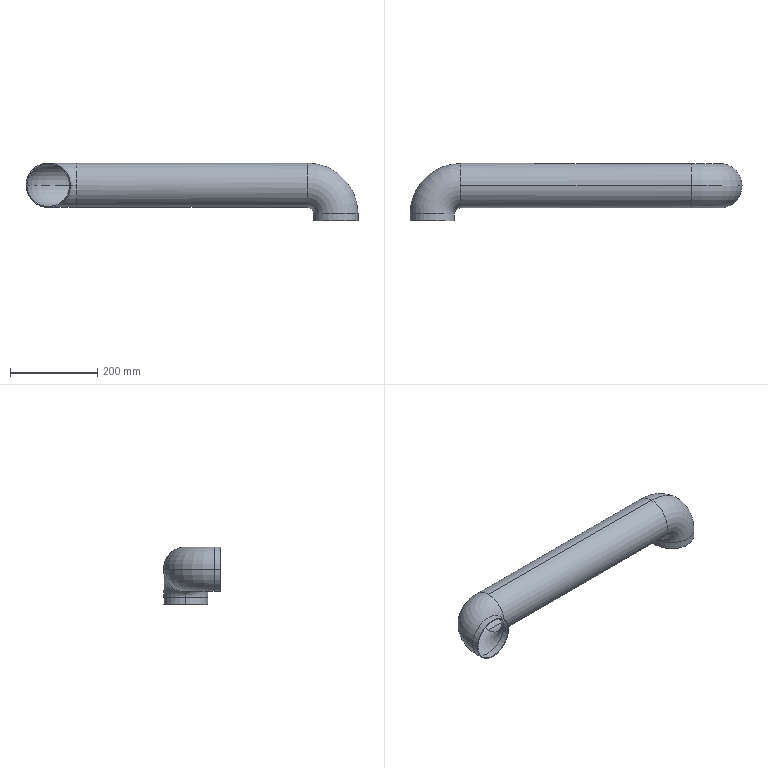Part | SolidWorks | features BaseBody 1 | 1 solid | 22 faces | box 761.5 x 131 x 133 mm | volume 481106 mm3 | cylinder 12 | torus 8 | plane 2 | commonest cylinder face diameters 98 x6 102 x6
STEP:
#1=CARTESIAN_POINT('',(65.,80.,51.));
#2=VERTEX_POINT('',#1);
#3=CARTESIAN_POINT('',(65.,131.,0.));
#4=VERTEX_POINT('',#3);
#5=CARTESIAN_POINT('',(65.,80.,0.));
#6=DIRECTION('',(-1.,0.,0.));
#7=DIRECTION('',(0.,0.,1.));
#8=AXIS2_PLACEMENT_3D('',#5,#6,#7);
#9=CIRCLE('',#8,51.);
#10=EDGE_CURVE('',#2,#4,#9,.T.);
#11=ORIENTED_EDGE('',*,*,#10,.T.);
#12=CARTESIAN_POINT('',(-51.,15.,0.));
#13=VERTEX_POINT('',#12);
#14=CARTESIAN_POINT('',(65.,15.,0.));
#15=DIRECTION('',(0.,0.,1.));
#16=DIRECTION('',(1.,0.,0.));
#17=AXIS2_PLACEMENT_3D('',#14,#15,#16);
#18=CIRCLE('',#17,116.);
#19=EDGE_CURVE('',#4,#13,#18,.T.);
#20=ORIENTED_EDGE('',*,*,#19,.T.);
#21=CARTESIAN_POINT('',(51.,15.,0.));
#22=VERTEX_POINT('',#21);
#23=CARTESIAN_POINT('',(0.,15.,0.));
#24=DIRECTION('',(0.,-1.,0.));
#25=DIRECTION('',(0.,0.,1.));
#26=AXIS2_PLACEMENT_3D('',#23,#24,#25);
#27=CIRCLE('',#26,51.);
#28=EDGE_CURVE('',#22,#13,#27,.T.);
#29=ORIENTED_EDGE('',*,*,#28,.F.);
#30=CARTESIAN_POINT('',(65.,29.,0.));
#31=VERTEX_POINT('',#30);
#32=CARTESIAN_POINT('',(65.,15.,0.));
#33=DIRECTION('',(0.,0.,1.));
#34=DIRECTION('',(1.,0.,0.));
#35=AXIS2_PLACEMENT_3D('',#32,#33,#34);
#36=CIRCLE('',#35,14.);
#37=EDGE_CURVE('',#31,#22,#36,.T.);
#38=ORIENTED_EDGE('',*,*,#37,.F.);
#39=CARTESIAN_POINT('',(65.,80.,0.));
#40=DIRECTION('',(-1.,0.,0.));
#41=DIRECTION('',(0.,0.,1.));
#42=AXIS2_PLACEMENT_3D('',#39,#40,#41);
#43=CIRCLE('',#42,51.);
#44=EDGE_CURVE('',#31,#2,#43,.T.);
#45=ORIENTED_EDGE('',*,*,#44,.T.);
#46=EDGE_LOOP('',(#11,#20,#29,#38,#45));
#47=FACE_OUTER_BOUND('',#46,.T.);
#48=CARTESIAN_POINT('',(65.,15.,0.));
#49=DIRECTION('',(0.,0.,1.));
#50=DIRECTION('',(1.,0.,0.));
#51=AXIS2_PLACEMENT_3D('',#48,#49,#50);
#52=TOROIDAL_SURFACE('',#51,65.,51.);
#53=ADVANCED_FACE('',(#47),#52,.T.);
#54=CARTESIAN_POINT('',(65.,129.,0.));
#55=VERTEX_POINT('',#54);
#56=CARTESIAN_POINT('',(65.,80.,-49.));
#57=VERTEX_POINT('',#56);
#58=CARTESIAN_POINT('',(65.,80.,0.));
#59=DIRECTION('',(-1.,0.,0.));
#60=DIRECTION('',(0.,0.,1.));
#61=AXIS2_PLACEMENT_3D('',#58,#59,#60);
#62=CIRCLE('',#61,49.);
#63=EDGE_CURVE('',#55,#57,#62,.T.);
#64=ORIENTED_EDGE('',*,*,#63,.F.);
#65=CARTESIAN_POINT('',(-49.,15.,0.));
#66=VERTEX_POINT('',#65);
#67=CARTESIAN_POINT('',(65.,15.,0.));
#68=DIRECTION('',(0.,0.,1.));
#69=DIRECTION('',(1.,0.,0.));
#70=AXIS2_PLACEMENT_3D('',#67,#68,#69);
#71=CIRCLE('',#70,114.);
#72=EDGE_CURVE('',#55,#66,#71,.T.);
#73=ORIENTED_EDGE('',*,*,#72,.T.);
#74=CARTESIAN_POINT('',(49.,15.,0.));
#75=VERTEX_POINT('',#74);
#76=CARTESIAN_POINT('',(0.,15.,0.));
#77=DIRECTION('',(0.,-1.,0.));
#78=DIRECTION('',(0.,0.,1.));
#79=AXIS2_PLACEMENT_3D('',#76,#77,#78);
#80=CIRCLE('',#79,49.);
#81=EDGE_CURVE('',#66,#75,#80,.T.);
#82=ORIENTED_EDGE('',*,*,#81,.T.);
#83=CARTESIAN_POINT('',(65.,31.,0.));
#84=VERTEX_POINT('',#83);
#85=CARTESIAN_POINT('',(65.,15.,0.));
#86=DIRECTION('',(0.,0.,1.));
#87=DIRECTION('',(1.,0.,0.));
#88=AXIS2_PLACEMENT_3D('',#85,#86,#87);
#89=CIRCLE('',#88,16.);
#90=EDGE_CURVE('',#84,#75,#89,.T.);
#91=ORIENTED_EDGE('',*,*,#90,.F.);
#92=CARTESIAN_POINT('',(65.,80.,0.));
#93=DIRECTION('',(-1.,0.,0.));
#94=DIRECTION('',(0.,0.,1.));
#95=AXIS2_PLACEMENT_3D('',#92,#93,#94);
#96=CIRCLE('',#95,49.);
#97=EDGE_CURVE('',#57,#84,#96,.T.);
#98=ORIENTED_EDGE('',*,*,#97,.F.);
#99=EDGE_LOOP('',(#64,#73,#82,#91,#98));
#100=FACE_OUTER_BOUND('',#99,.T.);
#101=CARTESIAN_POINT('',(65.,15.,0.));
#102=DIRECTION('',(0.,0.,1.));
#103=DIRECTION('',(1.,0.,0.));
#104=AXIS2_PLACEMENT_3D('',#101,#102,#103);
#105=TOROIDAL_SURFACE('',#104,65.,49.);
#106=ADVANCED_FACE('',(#100),#105,.F.);
#107=CARTESIAN_POINT('',(608.5,80.,-65.));
#108=VERTEX_POINT('',#107);
#109=CARTESIAN_POINT('',(710.5,80.,-65.));
#110=VERTEX_POINT('',#109);
#111=CARTESIAN_POINT('',(659.5,80.,-65.));
#112=DIRECTION('',(0.,0.,1.));
#113=DIRECTION('',(1.,0.,0.));
#114=AXIS2_PLACEMENT_3D('',#111,#112,#113);
#115=CIRCLE('',#114,51.);
#116=EDGE_CURVE('',#108,#110,#115,.T.);
#117=ORIENTED_EDGE('',*,*,#116,.T.);
#118=CARTESIAN_POINT('',(594.5,80.,51.));
#119=VERTEX_POINT('',#118);
#120=CARTESIAN_POINT('',(594.5,80.,-65.));
#121=DIRECTION('',(0.,-1.,0.));
#122=DIRECTION('',(0.,0.,-1.));
#123=AXIS2_PLACEMENT_3D('',#120,#121,#122);
#124=CIRCLE('',#123,116.);
#125=EDGE_CURVE('',#110,#119,#124,.T.);
#126=ORIENTED_EDGE('',*,*,#125,.T.);
#127=CARTESIAN_POINT('',(594.5,80.,-51.));
#128=VERTEX_POINT('',#127);
#129=CARTESIAN_POINT('',(594.5,80.,0.));
#130=DIRECTION('',(-1.,0.,0.));
#131=DIRECTION('',(0.,0.,1.));
#132=AXIS2_PLACEMENT_3D('',#129,#130,#131);
#133=CIRCLE('',#132,51.);
#134=EDGE_CURVE('',#128,#119,#133,.T.);
#135=ORIENTED_EDGE('',*,*,#134,.F.);
#136=CARTESIAN_POINT('',(594.5,80.,-65.));
#137=DIRECTION('',(0.,-1.,0.));
#138=DIRECTION('',(0.,0.,-1.));
#139=AXIS2_PLACEMENT_3D('',#136,#137,#138);
#140=CIRCLE('',#139,14.);
#141=EDGE_CURVE('',#108,#128,#140,.T.);
#142=ORIENTED_EDGE('',*,*,#141,.F.);
#143=EDGE_LOOP('',(#117,#126,#135,#142));
#144=FACE_OUTER_BOUND('',#143,.T.);
#145=CARTESIAN_POINT('',(594.5,80.,-65.));
#146=DIRECTION('',(0.,-1.,0.));
#147=DIRECTION('',(0.,0.,-1.));
#148=AXIS2_PLACEMENT_3D('',#145,#146,#147);
#149=TOROIDAL_SURFACE('',#148,65.,51.);
#150=ADVANCED_FACE('',(#144),#149,.T.);
#151=CARTESIAN_POINT('',(708.5,80.,-65.));
#152=VERTEX_POINT('',#151);
#153=CARTESIAN_POINT('',(610.5,80.,-65.));
#154=VERTEX_POINT('',#153);
#155=CARTESIAN_POINT('',(659.5,80.,-65.));
#156=DIRECTION('',(0.,0.,1.));
#157=DIRECTION('',(1.,0.,0.));
#158=AXIS2_PLACEMENT_3D('',#155,#156,#157);
#159=CIRCLE('',#158,49.);
#160=EDGE_CURVE('',#152,#154,#159,.T.);
#161=ORIENTED_EDGE('',*,*,#160,.F.);
#162=CARTESIAN_POINT('',(594.5,80.,49.));
#163=VERTEX_POINT('',#162);
#164=CARTESIAN_POINT('',(594.5,80.,-65.));
#165=DIRECTION('',(0.,-1.,0.));
#166=DIRECTION('',(0.,0.,-1.));
#167=AXIS2_PLACEMENT_3D('',#164,#165,#166);
#168=CIRCLE('',#167,114.);
#169=EDGE_CURVE('',#152,#163,#168,.T.);
#170=ORIENTED_EDGE('',*,*,#169,.T.);
#171=CARTESIAN_POINT('',(594.5,80.,-49.));
#172=VERTEX_POINT('',#171);
#173=CARTESIAN_POINT('',(594.5,80.,0.));
#174=DIRECTION('',(-1.,0.,0.));
#175=DIRECTION('',(0.,0.,1.));
#176=AXIS2_PLACEMENT_3D('',#173,#174,#175);
#177=CIRCLE('',#176,49.);
#178=EDGE_CURVE('',#163,#172,#177,.T.);
#179=ORIENTED_EDGE('',*,*,#178,.T.);
#180=CARTESIAN_POINT('',(594.5,80.,-65.));
#181=DIRECTION('',(0.,-1.,0.));
#182=DIRECTION('',(0.,0.,-1.));
#183=AXIS2_PLACEMENT_3D('',#180,#181,#182);
#184=CIRCLE('',#183,16.);
#185=EDGE_CURVE('',#154,#172,#184,.T.);
#186=ORIENTED_EDGE('',*,*,#185,.F.);
#187=EDGE_LOOP('',(#161,#170,#179,#186));
#188=FACE_OUTER_BOUND('',#187,.T.);
#189=CARTESIAN_POINT('',(594.5,80.,-65.));
#190=DIRECTION('',(0.,-1.,0.));
#191=DIRECTION('',(0.,0.,-1.));
#192=AXIS2_PLACEMENT_3D('',#189,#190,#191);
#193=TOROIDAL_SURFACE('',#192,65.,49.);
#194=ADVANCED_FACE('',(#188),#193,.F.);
#195=ORIENTED_EDGE('',*,*,#28,.T.);
#196=CARTESIAN_POINT('',(-51.,0.,0.));
#197=VERTEX_POINT('',#196);
#198=CARTESIAN_POINT('',(-51.,15.,0.));
#199=DIRECTION('',(0.,-1.,0.));
#200=VECTOR('',#199,1000.);
#201=LINE('',#198,#200);
#202=EDGE_CURVE('',#13,#197,#201,.T.);
#203=ORIENTED_EDGE('',*,*,#202,.T.);
#204=CARTESIAN_POINT('',(51.,0.,0.));
#205=VERTEX_POINT('',#204);
#206=CARTESIAN_POINT('',(0.,0.,0.));
#207=DIRECTION('',(0.,-1.,0.));
#208=DIRECTION('',(0.,0.,1.));
#209=AXIS2_PLACEMENT_3D('',#206,#207,#208);
#210=CIRCLE('',#209,51.);
#211=EDGE_CURVE('',#205,#197,#210,.T.);
#212=ORIENTED_EDGE('',*,*,#211,.F.);
#213=CARTESIAN_POINT('',(51.,15.,0.));
#214=DIRECTION('',(0.,-1.,0.));
#215=VECTOR('',#214,1000.);
#216=LINE('',#213,#215);
#217=EDGE_CURVE('',#22,#205,#216,.T.);
#218=ORIENTED_EDGE('',*,*,#217,.F.);
#219=EDGE_LOOP('',(#195,#203,#212,#218));
#220=FACE_OUTER_BOUND('',#219,.T.);
#221=CARTESIAN_POINT('',(0.,15.,0.));
#222=DIRECTION('',(0.,-1.,0.));
#223=DIRECTION('',(1.,0.,0.));
#224=AXIS2_PLACEMENT_3D('',#221,#222,#223);
#225=CYLINDRICAL_SURFACE('',#224,51.);
#226=ADVANCED_FACE('',(#220),#225,.T.);
#227=ORIENTED_EDGE('',*,*,#81,.F.);
#228=CARTESIAN_POINT('',(-49.,0.,0.));
#229=VERTEX_POINT('',#228);
#230=CARTESIAN_POINT('',(-49.,15.,0.));
#231=DIRECTION('',(0.,-1.,0.));
#232=VECTOR('',#231,1000.);
#233=LINE('',#230,#232);
#234=EDGE_CURVE('',#66,#229,#233,.T.);
#235=ORIENTED_EDGE('',*,*,#234,.T.);
#236=CARTESIAN_POINT('',(49.,0.,0.));
#237=VERTEX_POINT('',#236);
#238=CARTESIAN_POINT('',(0.,0.,0.));
#239=DIRECTION('',(0.,-1.,0.));
#240=DIRECTION('',(0.,0.,1.));
#241=AXIS2_PLACEMENT_3D('',#238,#239,#240);
#242=CIRCLE('',#241,49.);
#243=EDGE_CURVE('',#229,#237,#242,.T.);
#244=ORIENTED_EDGE('',*,*,#243,.T.);
#245=CARTESIAN_POINT('',(49.,15.,0.));
#246=DIRECTION('',(0.,-1.,0.));
#247=VECTOR('',#246,1000.);
#248=LINE('',#245,#247);
#249=EDGE_CURVE('',#75,#237,#248,.T.);
#250=ORIENTED_EDGE('',*,*,#249,.F.);
#251=EDGE_LOOP('',(#227,#235,#244,#250));
#252=FACE_OUTER_BOUND('',#251,.T.);
#253=CARTESIAN_POINT('',(0.,15.,0.));
#254=DIRECTION('',(0.,-1.,0.));
#255=DIRECTION('',(1.,0.,0.));
#256=AXIS2_PLACEMENT_3D('',#253,#254,#255);
#257=CYLINDRICAL_SURFACE('',#256,49.);
#258=ADVANCED_FACE('',(#252),#257,.F.);
#259=CARTESIAN_POINT('',(594.5,80.,0.));
#260=DIRECTION('',(-1.,0.,0.));
#261=DIRECTION('',(0.,0.,1.));
#262=AXIS2_PLACEMENT_3D('',#259,#260,#261);
#263=CIRCLE('',#262,51.);
#264=EDGE_CURVE('',#119,#128,#263,.T.);
#265=ORIENTED_EDGE('',*,*,#264,.T.);
#266=CARTESIAN_POINT('',(65.,80.,-51.));
#267=VERTEX_POINT('',#266);
#268=CARTESIAN_POINT('',(594.5,80.,-51.));
#269=DIRECTION('',(-1.,0.,0.));
#270=VECTOR('',#269,1000.);
#271=LINE('',#268,#270);
#272=EDGE_CURVE('',#128,#267,#271,.T.);
#273=ORIENTED_EDGE('',*,*,#272,.T.);
#274=CARTESIAN_POINT('',(65.,80.,0.));
#275=DIRECTION('',(-1.,0.,0.));
#276=DIRECTION('',(0.,0.,1.));
#277=AXIS2_PLACEMENT_3D('',#274,#275,#276);
#278=CIRCLE('',#277,51.);
#279=EDGE_CURVE('',#4,#267,#278,.T.);
#280=ORIENTED_EDGE('',*,*,#279,.F.);
#281=ORIENTED_EDGE('',*,*,#10,.F.);
#282=CARTESIAN_POINT('',(594.5,80.,51.));
#283=DIRECTION('',(-1.,0.,0.));
#284=VECTOR('',#283,1000.);
#285=LINE('',#282,#284);
#286=EDGE_CURVE('',#119,#2,#285,.T.);
#287=ORIENTED_EDGE('',*,*,#286,.F.);
#288=EDGE_LOOP('',(#265,#273,#280,#281,#287));
#289=FACE_OUTER_BOUND('',#288,.T.);
#290=CARTESIAN_POINT('',(594.5,80.,0.));
#291=DIRECTION('',(-1.,0.,0.));
#292=DIRECTION('',(0.,0.,1.));
#293=AXIS2_PLACEMENT_3D('',#290,#291,#292);
#294=CYLINDRICAL_SURFACE('',#293,51.);
#295=ADVANCED_FACE('',(#289),#294,.T.);
#296=CARTESIAN_POINT('',(594.5,80.,0.));
#297=DIRECTION('',(-1.,0.,0.));
#298=DIRECTION('',(0.,0.,1.));
#299=AXIS2_PLACEMENT_3D('',#296,#297,#298);
#300=CIRCLE('',#299,49.);
#301=EDGE_CURVE('',#172,#163,#300,.T.);
#302=ORIENTED_EDGE('',*,*,#301,.F.);
#303=CARTESIAN_POINT('',(594.5,80.,-49.));
#304=DIRECTION('',(-1.,0.,0.));
#305=VECTOR('',#304,1000.);
#306=LINE('',#303,#305);
#307=EDGE_CURVE('',#172,#57,#306,.T.);
#308=ORIENTED_EDGE('',*,*,#307,.T.);
#309=ORIENTED_EDGE('',*,*,#97,.T.);
#310=CARTESIAN_POINT('',(65.,80.,49.));
#311=VERTEX_POINT('',#310);
#312=CARTESIAN_POINT('',(65.,80.,0.));
#313=DIRECTION('',(-1.,0.,0.));
#314=DIRECTION('',(0.,0.,1.));
#315=AXIS2_PLACEMENT_3D('',#312,#313,#314);
#316=CIRCLE('',#315,49.);
#317=EDGE_CURVE('',#84,#311,#316,.T.);
#318=ORIENTED_EDGE('',*,*,#317,.T.);
#319=CARTESIAN_POINT('',(594.5,80.,49.));
#320=DIRECTION('',(-1.,0.,0.));
#321=VECTOR('',#320,1000.);
#322=LINE('',#319,#321);
#323=EDGE_CURVE('',#163,#311,#322,.T.);
#324=ORIENTED_EDGE('',*,*,#323,.F.);
#325=EDGE_LOOP('',(#302,#308,#309,#318,#324));
#326=FACE_OUTER_BOUND('',#325,.T.);
#327=CARTESIAN_POINT('',(594.5,80.,0.));
#328=DIRECTION('',(-1.,0.,0.));
#329=DIRECTION('',(0.,0.,1.));
#330=AXIS2_PLACEMENT_3D('',#327,#328,#329);
#331=CYLINDRICAL_SURFACE('',#330,49.);
#332=ADVANCED_FACE('',(#326),#331,.F.);
#333=CARTESIAN_POINT('',(659.5,80.,-65.));
#334=DIRECTION('',(0.,0.,1.));
#335=DIRECTION('',(1.,0.,0.));
#336=AXIS2_PLACEMENT_3D('',#333,#334,#335);
#337=CIRCLE('',#336,49.);
#338=EDGE_CURVE('',#154,#152,#337,.T.);
#339=ORIENTED_EDGE('',*,*,#338,.T.);
#340=CARTESIAN_POINT('',(708.5,80.,-82.));
#341=VERTEX_POINT('',#340);
#342=CARTESIAN_POINT('',(708.5,80.,-65.));
#343=DIRECTION('',(0.,0.,-1.));
#344=VECTOR('',#343,1000.);
#345=LINE('',#342,#344);
#346=EDGE_CURVE('',#152,#341,#345,.T.);
#347=ORIENTED_EDGE('',*,*,#346,.T.);
#348=CARTESIAN_POINT('',(610.5,80.,-82.));
#349=VERTEX_POINT('',#348);
#350=CARTESIAN_POINT('',(659.5,80.,-82.));
#351=DIRECTION('',(0.,0.,1.));
#352=DIRECTION('',(1.,0.,0.));
#353=AXIS2_PLACEMENT_3D('',#350,#351,#352);
#354=CIRCLE('',#353,49.);
#355=EDGE_CURVE('',#349,#341,#354,.T.);
#356=ORIENTED_EDGE('',*,*,#355,.F.);
#357=CARTESIAN_POINT('',(610.5,80.,-65.));
#358=DIRECTION('',(0.,0.,-1.));
#359=VECTOR('',#358,1000.);
#360=LINE('',#357,#359);
#361=EDGE_CURVE('',#154,#349,#360,.T.);
#362=ORIENTED_EDGE('',*,*,#361,.F.);
#363=EDGE_LOOP('',(#339,#347,#356,#362));
#364=FACE_OUTER_BOUND('',#363,.T.);
#365=CARTESIAN_POINT('',(659.5,80.,-65.));
#366=DIRECTION('',(0.,0.,-1.));
#367=DIRECTION('',(-1.,0.,0.));
#368=AXIS2_PLACEMENT_3D('',#365,#366,#367);
#369=CYLINDRICAL_SURFACE('',#368,49.);
#370=ADVANCED_FACE('',(#364),#369,.F.);
#371=CARTESIAN_POINT('',(659.5,80.,-65.));
#372=DIRECTION('',(0.,0.,1.));
#373=DIRECTION('',(1.,0.,0.));
#374=AXIS2_PLACEMENT_3D('',#371,#372,#373);
#375=CIRCLE('',#374,51.);
#376=EDGE_CURVE('',#110,#108,#375,.T.);
#377=ORIENTED_EDGE('',*,*,#376,.F.);
#378=CARTESIAN_POINT('',(710.5,80.,-82.));
#379=VERTEX_POINT('',#378);
#380=CARTESIAN_POINT('',(710.5,80.,-65.));
#381=DIRECTION('',(0.,0.,-1.));
#382=VECTOR('',#381,1000.);
#383=LINE('',#380,#382);
#384=EDGE_CURVE('',#110,#379,#383,.T.);
#385=ORIENTED_EDGE('',*,*,#384,.T.);
#386=CARTESIAN_POINT('',(608.5,80.,-82.));
#387=VERTEX_POINT('',#386);
#388=CARTESIAN_POINT('',(659.5,80.,-82.));
#389=DIRECTION('',(0.,0.,1.));
#390=DIRECTION('',(1.,0.,0.));
#391=AXIS2_PLACEMENT_3D('',#388,#389,#390);
#392=CIRCLE('',#391,51.);
#393=EDGE_CURVE('',#379,#387,#392,.T.);
#394=ORIENTED_EDGE('',*,*,#393,.T.);
#395=CARTESIAN_POINT('',(608.5,80.,-65.));
#396=DIRECTION('',(0.,0.,-1.));
#397=VECTOR('',#396,1000.);
#398=LINE('',#395,#397);
#399=EDGE_CURVE('',#108,#387,#398,.T.);
#400=ORIENTED_EDGE('',*,*,#399,.F.);
#401=EDGE_LOOP('',(#377,#385,#394,#400));
#402=FACE_OUTER_BOUND('',#401,.T.);
#403=CARTESIAN_POINT('',(659.5,80.,-65.));
#404=DIRECTION('',(0.,0.,-1.));
#405=DIRECTION('',(-1.,0.,0.));
#406=AXIS2_PLACEMENT_3D('',#403,#404,#405);
#407=CYLINDRICAL_SURFACE('',#406,51.);
#408=ADVANCED_FACE('',(#402),#407,.T.);
#409=CARTESIAN_POINT('',(659.5,80.,-82.));
#410=DIRECTION('',(0.,0.,1.));
#411=DIRECTION('',(1.,0.,0.));
#412=AXIS2_PLACEMENT_3D('',#409,#410,#411);
#413=CIRCLE('',#412,51.);
#414=EDGE_CURVE('',#387,#379,#413,.T.);
#415=ORIENTED_EDGE('',*,*,#414,.F.);
#416=ORIENTED_EDGE('',*,*,#393,.F.);
#417=EDGE_LOOP('',(#415,#416));
#418=FACE_OUTER_BOUND('',#417,.T.);
#419=ORIENTED_EDGE('',*,*,#355,.T.);
#420=CARTESIAN_POINT('',(659.5,80.,-82.));
#421=DIRECTION('',(0.,0.,1.));
#422=DIRECTION('',(1.,0.,0.));
#423=AXIS2_PLACEMENT_3D('',#420,#421,#422);
#424=CIRCLE('',#423,49.);
#425=EDGE_CURVE('',#341,#349,#424,.T.);
#426=ORIENTED_EDGE('',*,*,#425,.T.);
#427=EDGE_LOOP('',(#419,#426));
#428=FACE_BOUND('',#427,.T.);
#429=CARTESIAN_POINT('',(659.5,80.,-82.));
#430=DIRECTION('',(0.,0.,1.));
#431=DIRECTION('',(1.,0.,0.));
#432=AXIS2_PLACEMENT_3D('',#429,#430,#431);
#433=PLANE('',#432);
#434=ADVANCED_FACE('',(#418,#428),#433,.F.);
#435=ORIENTED_EDGE('',*,*,#211,.T.);
#436=CARTESIAN_POINT('',(0.,0.,0.));
#437=DIRECTION('',(0.,-1.,0.));
#438=DIRECTION('',(0.,0.,1.));
#439=AXIS2_PLACEMENT_3D('',#436,#437,#438);
#440=CIRCLE('',#439,51.);
#441=EDGE_CURVE('',#197,#205,#440,.T.);
#442=ORIENTED_EDGE('',*,*,#441,.T.);
#443=EDGE_LOOP('',(#435,#442));
#444=FACE_OUTER_BOUND('',#443,.T.);
#445=CARTESIAN_POINT('',(0.,0.,0.));
#446=DIRECTION('',(0.,-1.,0.));
#447=DIRECTION('',(0.,0.,1.));
#448=AXIS2_PLACEMENT_3D('',#445,#446,#447);
#449=CIRCLE('',#448,49.);
#450=EDGE_CURVE('',#237,#229,#449,.T.);
#451=ORIENTED_EDGE('',*,*,#450,.F.);
#452=ORIENTED_EDGE('',*,*,#243,.F.);
#453=EDGE_LOOP('',(#451,#452));
#454=FACE_BOUND('',#453,.T.);
#455=CARTESIAN_POINT('',(0.,0.,0.));
#456=DIRECTION('',(0.,-1.,0.));
#457=DIRECTION('',(0.,0.,-1.));
#458=AXIS2_PLACEMENT_3D('',#455,#456,#457);
#459=PLANE('',#458);
#460=ADVANCED_FACE('',(#444,#454),#459,.T.);
#461=ORIENTED_EDGE('',*,*,#384,.F.);
#462=ORIENTED_EDGE('',*,*,#116,.F.);
#463=ORIENTED_EDGE('',*,*,#399,.T.);
#464=ORIENTED_EDGE('',*,*,#414,.T.);
#465=EDGE_LOOP('',(#461,#462,#463,#464));
#466=FACE_OUTER_BOUND('',#465,.T.);
#467=CARTESIAN_POINT('',(659.5,80.,-65.));
#468=DIRECTION('',(0.,0.,-1.));
#469=DIRECTION('',(-1.,0.,0.));
#470=AXIS2_PLACEMENT_3D('',#467,#468,#469);
#471=CYLINDRICAL_SURFACE('',#470,51.);
#472=ADVANCED_FACE('',(#466),#471,.T.);
#473=ORIENTED_EDGE('',*,*,#346,.F.);
#474=ORIENTED_EDGE('',*,*,#160,.T.);
#475=ORIENTED_EDGE('',*,*,#361,.T.);
#476=ORIENTED_EDGE('',*,*,#425,.F.);
#477=EDGE_LOOP('',(#473,#474,#475,#476));
#478=FACE_OUTER_BOUND('',#477,.T.);
#479=CARTESIAN_POINT('',(659.5,80.,-65.));
#480=DIRECTION('',(0.,0.,-1.));
#481=DIRECTION('',(-1.,0.,0.));
#482=AXIS2_PLACEMENT_3D('',#479,#480,#481);
#483=CYLINDRICAL_SURFACE('',#482,49.);
#484=ADVANCED_FACE('',(#478),#483,.F.);
#485=ORIENTED_EDGE('',*,*,#169,.F.);
#486=ORIENTED_EDGE('',*,*,#338,.F.);
#487=ORIENTED_EDGE('',*,*,#185,.T.);
#488=ORIENTED_EDGE('',*,*,#301,.T.);
#489=EDGE_LOOP('',(#485,#486,#487,#488));
#490=FACE_OUTER_BOUND('',#489,.T.);
#491=CARTESIAN_POINT('',(594.5,80.,-65.));
#492=DIRECTION('',(0.,-1.,0.));
#493=DIRECTION('',(0.,0.,-1.));
#494=AXIS2_PLACEMENT_3D('',#491,#492,#493);
#495=TOROIDAL_SURFACE('',#494,65.,49.);
#496=ADVANCED_FACE('',(#490),#495,.F.);
#497=ORIENTED_EDGE('',*,*,#125,.F.);
#498=ORIENTED_EDGE('',*,*,#376,.T.);
#499=ORIENTED_EDGE('',*,*,#141,.T.);
#500=ORIENTED_EDGE('',*,*,#264,.F.);
#501=EDGE_LOOP('',(#497,#498,#499,#500));
#502=FACE_OUTER_BOUND('',#501,.T.);
#503=CARTESIAN_POINT('',(594.5,80.,-65.));
#504=DIRECTION('',(0.,-1.,0.));
#505=DIRECTION('',(0.,0.,-1.));
#506=AXIS2_PLACEMENT_3D('',#503,#504,#505);
#507=TOROIDAL_SURFACE('',#506,65.,51.);
#508=ADVANCED_FACE('',(#502),#507,.T.);
#509=ORIENTED_EDGE('',*,*,#307,.F.);
#510=ORIENTED_EDGE('',*,*,#178,.F.);
#511=ORIENTED_EDGE('',*,*,#323,.T.);
#512=CARTESIAN_POINT('',(65.,80.,0.));
#513=DIRECTION('',(-1.,0.,0.));
#514=DIRECTION('',(0.,0.,1.));
#515=AXIS2_PLACEMENT_3D('',#512,#513,#514);
#516=CIRCLE('',#515,49.);
#517=EDGE_CURVE('',#311,#55,#516,.T.);
#518=ORIENTED_EDGE('',*,*,#517,.T.);
#519=ORIENTED_EDGE('',*,*,#63,.T.);
#520=EDGE_LOOP('',(#509,#510,#511,#518,#519));
#521=FACE_OUTER_BOUND('',#520,.T.);
#522=CARTESIAN_POINT('',(594.5,80.,0.));
#523=DIRECTION('',(-1.,0.,0.));
#524=DIRECTION('',(0.,0.,1.));
#525=AXIS2_PLACEMENT_3D('',#522,#523,#524);
#526=CYLINDRICAL_SURFACE('',#525,49.);
#527=ADVANCED_FACE('',(#521),#526,.F.);
#528=ORIENTED_EDGE('',*,*,#272,.F.);
#529=ORIENTED_EDGE('',*,*,#134,.T.);
#530=ORIENTED_EDGE('',*,*,#286,.T.);
#531=ORIENTED_EDGE('',*,*,#44,.F.);
#532=CARTESIAN_POINT('',(65.,80.,0.));
#533=DIRECTION('',(-1.,0.,0.));
#534=DIRECTION('',(0.,0.,1.));
#535=AXIS2_PLACEMENT_3D('',#532,#533,#534);
#536=CIRCLE('',#535,51.);
#537=EDGE_CURVE('',#267,#31,#536,.T.);
#538=ORIENTED_EDGE('',*,*,#537,.F.);
#539=EDGE_LOOP('',(#528,#529,#530,#531,#538));
#540=FACE_OUTER_BOUND('',#539,.T.);
#541=CARTESIAN_POINT('',(594.5,80.,0.));
#542=DIRECTION('',(-1.,0.,0.));
#543=DIRECTION('',(0.,0.,1.));
#544=AXIS2_PLACEMENT_3D('',#541,#542,#543);
#545=CYLINDRICAL_SURFACE('',#544,51.);
#546=ADVANCED_FACE('',(#540),#545,.T.);
#547=ORIENTED_EDGE('',*,*,#72,.F.);
#548=ORIENTED_EDGE('',*,*,#517,.F.);
#549=ORIENTED_EDGE('',*,*,#317,.F.);
#550=ORIENTED_EDGE('',*,*,#90,.T.);
#551=CARTESIAN_POINT('',(0.,15.,0.));
#552=DIRECTION('',(0.,-1.,0.));
#553=DIRECTION('',(0.,0.,1.));
#554=AXIS2_PLACEMENT_3D('',#551,#552,#553);
#555=CIRCLE('',#554,49.);
#556=EDGE_CURVE('',#75,#66,#555,.T.);
#557=ORIENTED_EDGE('',*,*,#556,.T.);
#558=EDGE_LOOP('',(#547,#548,#549,#550,#557));
#559=FACE_OUTER_BOUND('',#558,.T.);
#560=CARTESIAN_POINT('',(65.,15.,0.));
#561=DIRECTION('',(0.,0.,1.));
#562=DIRECTION('',(1.,0.,0.));
#563=AXIS2_PLACEMENT_3D('',#560,#561,#562);
#564=TOROIDAL_SURFACE('',#563,65.,49.);
#565=ADVANCED_FACE('',(#559),#564,.F.);
#566=ORIENTED_EDGE('',*,*,#19,.F.);
#567=ORIENTED_EDGE('',*,*,#279,.T.);
#568=ORIENTED_EDGE('',*,*,#537,.T.);
#569=ORIENTED_EDGE('',*,*,#37,.T.);
#570=CARTESIAN_POINT('',(0.,15.,0.));
#571=DIRECTION('',(0.,-1.,0.));
#572=DIRECTION('',(0.,0.,1.));
#573=AXIS2_PLACEMENT_3D('',#570,#571,#572);
#574=CIRCLE('',#573,51.);
#575=EDGE_CURVE('',#13,#22,#574,.T.);
#576=ORIENTED_EDGE('',*,*,#575,.F.);
#577=EDGE_LOOP('',(#566,#567,#568,#569,#576));
#578=FACE_OUTER_BOUND('',#577,.T.);
#579=CARTESIAN_POINT('',(65.,15.,0.));
#580=DIRECTION('',(0.,0.,1.));
#581=DIRECTION('',(1.,0.,0.));
#582=AXIS2_PLACEMENT_3D('',#579,#580,#581);
#583=TOROIDAL_SURFACE('',#582,65.,51.);
#584=ADVANCED_FACE('',(#578),#583,.T.);
#585=ORIENTED_EDGE('',*,*,#234,.F.);
#586=ORIENTED_EDGE('',*,*,#556,.F.);
#587=ORIENTED_EDGE('',*,*,#249,.T.);
#588=ORIENTED_EDGE('',*,*,#450,.T.);
#589=EDGE_LOOP('',(#585,#586,#587,#588));
#590=FACE_OUTER_BOUND('',#589,.T.);
#591=CARTESIAN_POINT('',(0.,15.,0.));
#592=DIRECTION('',(0.,-1.,0.));
#593=DIRECTION('',(1.,0.,0.));
#594=AXIS2_PLACEMENT_3D('',#591,#592,#593);
#595=CYLINDRICAL_SURFACE('',#594,49.);
#596=ADVANCED_FACE('',(#590),#595,.F.);
#597=ORIENTED_EDGE('',*,*,#202,.F.);
#598=ORIENTED_EDGE('',*,*,#575,.T.);
#599=ORIENTED_EDGE('',*,*,#217,.T.);
#600=ORIENTED_EDGE('',*,*,#441,.F.);
#601=EDGE_LOOP('',(#597,#598,#599,#600));
#602=FACE_OUTER_BOUND('',#601,.T.);
#603=CARTESIAN_POINT('',(0.,15.,0.));
#604=DIRECTION('',(0.,-1.,0.));
#605=DIRECTION('',(1.,0.,0.));
#606=AXIS2_PLACEMENT_3D('',#603,#604,#605);
#607=CYLINDRICAL_SURFACE('',#606,51.);
#608=ADVANCED_FACE('',(#602),#607,.T.);
#609=CLOSED_SHELL('',(#53,#106,#150,#194,#226,#258,#295,#332,#370,#408,#434,#460,#472,#484,#496,#508,#527,#546,#565,#584,#596,#608));
#610=MANIFOLD_SOLID_BREP('',#609);
#611=CARTESIAN_POINT('',(0.,0.,0.));
#612=DIRECTION('',(0.,0.,1.));
#613=DIRECTION('',(1.,0.,0.));
#614=AXIS2_PLACEMENT_3D('',#611,#612,#613);
#615=(LENGTH_UNIT()NAMED_UNIT(*)SI_UNIT(.MILLI.,.METRE.));
#616=UNCERTAINTY_MEASURE_WITH_UNIT(LENGTH_MEASURE(0.00001),#615,'','');
#617=(NAMED_UNIT(*)PLANE_ANGLE_UNIT()SI_UNIT($,.RADIAN.));
#618=(NAMED_UNIT(*)SI_UNIT($,.STERADIAN.)SOLID_ANGLE_UNIT());
#619=(GEOMETRIC_REPRESENTATION_CONTEXT(3)GLOBAL_UNCERTAINTY_ASSIGNED_CONTEXT((#616))GLOBAL_UNIT_ASSIGNED_CONTEXT((#615,#617,#618))REPRESENTATION_CONTEXT('',''));
#620=ADVANCED_BREP_SHAPE_REPRESENTATION('',(#610,#614),#619);